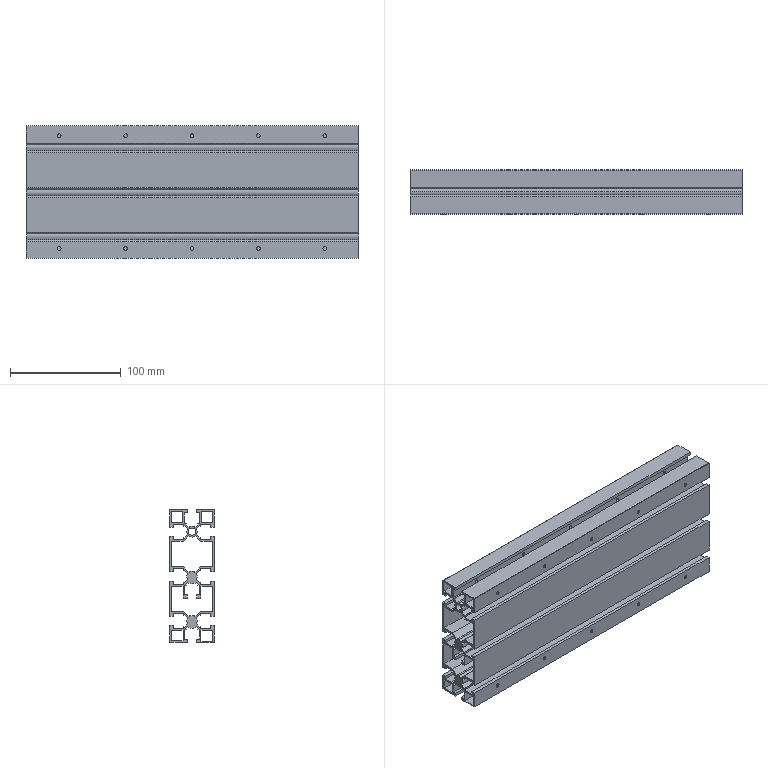Part | 1 solid | 239 faces | box 300 x 40 x 120 mm | volume 323531 mm3 | plane 160 | cylinder 79 | commonest cylinder face diameters 3.3 x60 9.6 x13 0.6 x2 6.6 x2 13.3 x2